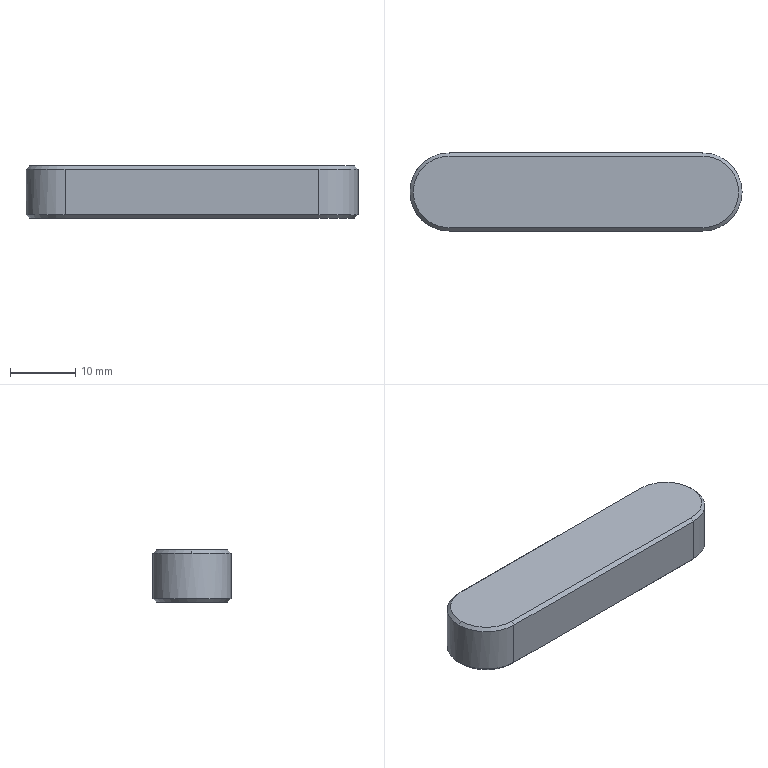Part | SolidWorks | features BaseBody 1 | 1 solid | 17 faces | box 51 x 12 x 8 mm | volume 4620 mm3 | plane 8 | cone 6 | cylinder 3 | commonest cylinder face diameters 12 x3
STEP:
#1=CARTESIAN_POINT('',(29.272,3.607,0.));
#2=VERTEX_POINT('',#1);
#3=CARTESIAN_POINT('',(34.772,9.107,0.));
#4=VERTEX_POINT('',#3);
#5=CARTESIAN_POINT('',(29.272,9.107,0.));
#6=DIRECTION('',(0.,0.,1.));
#7=DIRECTION('',(1.,0.,0.));
#8=AXIS2_PLACEMENT_3D('',#5,#6,#7);
#9=CIRCLE('',#8,5.5);
#10=EDGE_CURVE('',#2,#4,#9,.T.);
#11=ORIENTED_EDGE('',*,*,#10,.T.);
#12=CARTESIAN_POINT('',(35.272,9.107,0.5));
#13=VERTEX_POINT('',#12);
#14=CARTESIAN_POINT('',(35.272,9.107,0.5));
#15=DIRECTION('',(0.7071,0.,0.7071));
#16=VECTOR('',#15,1000.);
#17=LINE('',#14,#16);
#18=EDGE_CURVE('',#4,#13,#17,.T.);
#19=ORIENTED_EDGE('',*,*,#18,.T.);
#20=CARTESIAN_POINT('',(29.272,3.107,0.5));
#21=VERTEX_POINT('',#20);
#22=CARTESIAN_POINT('',(29.272,9.107,0.5));
#23=DIRECTION('',(0.,0.,-1.));
#24=DIRECTION('',(0.,1.,0.));
#25=AXIS2_PLACEMENT_3D('',#22,#23,#24);
#26=CIRCLE('',#25,6.);
#27=EDGE_CURVE('',#13,#21,#26,.T.);
#28=ORIENTED_EDGE('',*,*,#27,.T.);
#29=CARTESIAN_POINT('',(29.272,3.357,0.25));
#30=DIRECTION('',(0.,-0.7071,0.7071));
#31=VECTOR('',#30,1000.);
#32=LINE('',#29,#31);
#33=EDGE_CURVE('',#2,#21,#32,.T.);
#34=ORIENTED_EDGE('',*,*,#33,.F.);
#35=EDGE_LOOP('',(#11,#19,#28,#34));
#36=FACE_OUTER_BOUND('',#35,.T.);
#37=CARTESIAN_POINT('',(29.272,9.107,0.5));
#38=DIRECTION('',(0.,0.,1.));
#39=DIRECTION('',(1.,0.,0.));
#40=AXIS2_PLACEMENT_3D('',#37,#38,#39);
#41=CONICAL_SURFACE('',#40,6.,0.7854);
#42=ADVANCED_FACE('',(#36),#41,.T.);
#43=ORIENTED_EDGE('',*,*,#27,.F.);
#44=CARTESIAN_POINT('',(35.272,9.107,7.5));
#45=VERTEX_POINT('',#44);
#46=CARTESIAN_POINT('',(35.272,9.107,0.));
#47=DIRECTION('',(0.,0.,1.));
#48=VECTOR('',#47,1000.);
#49=LINE('',#46,#48);
#50=EDGE_CURVE('',#13,#45,#49,.T.);
#51=ORIENTED_EDGE('',*,*,#50,.T.);
#52=CARTESIAN_POINT('',(29.272,3.107,7.5));
#53=VERTEX_POINT('',#52);
#54=CARTESIAN_POINT('',(29.272,9.107,7.5));
#55=DIRECTION('',(0.,0.,-1.));
#56=DIRECTION('',(1.,0.,0.));
#57=AXIS2_PLACEMENT_3D('',#54,#55,#56);
#58=CIRCLE('',#57,6.);
#59=EDGE_CURVE('',#45,#53,#58,.T.);
#60=ORIENTED_EDGE('',*,*,#59,.T.);
#61=CARTESIAN_POINT('',(29.272,3.107,0.));
#62=DIRECTION('',(0.,0.,1.));
#63=VECTOR('',#62,1000.);
#64=LINE('',#61,#63);
#65=EDGE_CURVE('',#21,#53,#64,.T.);
#66=ORIENTED_EDGE('',*,*,#65,.F.);
#67=EDGE_LOOP('',(#43,#51,#60,#66));
#68=FACE_OUTER_BOUND('',#67,.T.);
#69=CARTESIAN_POINT('',(29.272,9.107,0.));
#70=DIRECTION('',(0.,0.,1.));
#71=DIRECTION('',(1.,0.,0.));
#72=AXIS2_PLACEMENT_3D('',#69,#70,#71);
#73=CYLINDRICAL_SURFACE('',#72,6.);
#74=ADVANCED_FACE('',(#68),#73,.T.);
#75=CARTESIAN_POINT('',(-9.728,3.607,8.));
#76=VERTEX_POINT('',#75);
#77=CARTESIAN_POINT('',(-15.228,9.107,8.));
#78=VERTEX_POINT('',#77);
#79=CARTESIAN_POINT('',(-9.728,9.107,8.));
#80=DIRECTION('',(0.,0.,-1.));
#81=DIRECTION('',(-1.,0.,0.));
#82=AXIS2_PLACEMENT_3D('',#79,#80,#81);
#83=CIRCLE('',#82,5.5);
#84=EDGE_CURVE('',#76,#78,#83,.T.);
#85=ORIENTED_EDGE('',*,*,#84,.T.);
#86=CARTESIAN_POINT('',(-15.728,9.107,7.5));
#87=VERTEX_POINT('',#86);
#88=CARTESIAN_POINT('',(-15.728,9.107,7.5));
#89=DIRECTION('',(-0.7071,0.,-0.7071));
#90=VECTOR('',#89,1000.);
#91=LINE('',#88,#90);
#92=EDGE_CURVE('',#78,#87,#91,.T.);
#93=ORIENTED_EDGE('',*,*,#92,.T.);
#94=CARTESIAN_POINT('',(-9.728,3.107,7.5));
#95=VERTEX_POINT('',#94);
#96=CARTESIAN_POINT('',(-9.728,9.107,7.5));
#97=DIRECTION('',(0.,0.,-1.));
#98=DIRECTION('',(1.,0.,0.));
#99=AXIS2_PLACEMENT_3D('',#96,#97,#98);
#100=CIRCLE('',#99,6.);
#101=EDGE_CURVE('',#95,#87,#100,.T.);
#102=ORIENTED_EDGE('',*,*,#101,.F.);
#103=CARTESIAN_POINT('',(-9.728,3.357,7.75));
#104=DIRECTION('',(0.,-0.7071,-0.7071));
#105=VECTOR('',#104,1000.);
#106=LINE('',#103,#105);
#107=EDGE_CURVE('',#76,#95,#106,.T.);
#108=ORIENTED_EDGE('',*,*,#107,.F.);
#109=EDGE_LOOP('',(#85,#93,#102,#108));
#110=FACE_OUTER_BOUND('',#109,.T.);
#111=CARTESIAN_POINT('',(-9.728,9.107,7.5));
#112=DIRECTION('',(0.,0.,-1.));
#113=DIRECTION('',(-1.,0.,0.));
#114=AXIS2_PLACEMENT_3D('',#111,#112,#113);
#115=CONICAL_SURFACE('',#114,6.,0.7854);
#116=ADVANCED_FACE('',(#110),#115,.T.);
#117=CARTESIAN_POINT('',(-9.728,14.607,0.));
#118=VERTEX_POINT('',#117);
#119=CARTESIAN_POINT('',(-9.728,3.607,0.));
#120=VERTEX_POINT('',#119);
#121=CARTESIAN_POINT('',(-9.728,9.107,0.));
#122=DIRECTION('',(0.,0.,1.));
#123=DIRECTION('',(1.,0.,0.));
#124=AXIS2_PLACEMENT_3D('',#121,#122,#123);
#125=CIRCLE('',#124,5.5);
#126=EDGE_CURVE('',#118,#120,#125,.T.);
#127=ORIENTED_EDGE('',*,*,#126,.F.);
#128=CARTESIAN_POINT('',(29.272,14.607,0.));
#129=VERTEX_POINT('',#128);
#130=CARTESIAN_POINT('',(9.772,14.607,0.));
#131=DIRECTION('',(-1.,0.,0.));
#132=VECTOR('',#131,1000.);
#133=LINE('',#130,#132);
#134=EDGE_CURVE('',#129,#118,#133,.T.);
#135=ORIENTED_EDGE('',*,*,#134,.F.);
#136=CARTESIAN_POINT('',(29.272,9.107,0.));
#137=DIRECTION('',(0.,0.,1.));
#138=DIRECTION('',(1.,0.,0.));
#139=AXIS2_PLACEMENT_3D('',#136,#137,#138);
#140=CIRCLE('',#139,5.5);
#141=EDGE_CURVE('',#4,#129,#140,.T.);
#142=ORIENTED_EDGE('',*,*,#141,.F.);
#143=ORIENTED_EDGE('',*,*,#10,.F.);
#144=CARTESIAN_POINT('',(9.772,3.607,0.));
#145=DIRECTION('',(1.,0.,0.));
#146=VECTOR('',#145,1000.);
#147=LINE('',#144,#146);
#148=EDGE_CURVE('',#120,#2,#147,.T.);
#149=ORIENTED_EDGE('',*,*,#148,.F.);
#150=EDGE_LOOP('',(#127,#135,#142,#143,#149));
#151=FACE_OUTER_BOUND('',#150,.T.);
#152=CARTESIAN_POINT('',(9.772,9.107,0.));
#153=DIRECTION('',(0.,0.,1.));
#154=DIRECTION('',(1.,0.,0.));
#155=AXIS2_PLACEMENT_3D('',#152,#153,#154);
#156=PLANE('',#155);
#157=ADVANCED_FACE('',(#151),#156,.F.);
#158=CARTESIAN_POINT('',(-9.728,3.107,0.5));
#159=VERTEX_POINT('',#158);
#160=CARTESIAN_POINT('',(-9.728,3.357,0.25));
#161=DIRECTION('',(0.,0.7071,-0.7071));
#162=VECTOR('',#161,1000.);
#163=LINE('',#160,#162);
#164=EDGE_CURVE('',#159,#120,#163,.T.);
#165=ORIENTED_EDGE('',*,*,#164,.T.);
#166=ORIENTED_EDGE('',*,*,#148,.T.);
#167=ORIENTED_EDGE('',*,*,#33,.T.);
#168=CARTESIAN_POINT('',(19.522,3.107,0.5));
#169=DIRECTION('',(-1.,0.,0.));
#170=VECTOR('',#169,1000.);
#171=LINE('',#168,#170);
#172=EDGE_CURVE('',#21,#159,#171,.T.);
#173=ORIENTED_EDGE('',*,*,#172,.T.);
#174=EDGE_LOOP('',(#165,#166,#167,#173));
#175=FACE_OUTER_BOUND('',#174,.T.);
#176=CARTESIAN_POINT('',(19.522,3.357,0.25));
#177=DIRECTION('',(0.,-0.7071,-0.7071));
#178=DIRECTION('',(0.,0.7071,-0.7071));
#179=AXIS2_PLACEMENT_3D('',#176,#177,#178);
#180=PLANE('',#179);
#181=ADVANCED_FACE('',(#175),#180,.T.);
#182=ORIENTED_EDGE('',*,*,#164,.F.);
#183=CARTESIAN_POINT('',(-9.728,15.107,0.5));
#184=VERTEX_POINT('',#183);
#185=CARTESIAN_POINT('',(-9.728,9.107,0.5));
#186=DIRECTION('',(0.,0.,-1.));
#187=DIRECTION('',(0.,-1.,0.));
#188=AXIS2_PLACEMENT_3D('',#185,#186,#187);
#189=CIRCLE('',#188,6.);
#190=EDGE_CURVE('',#159,#184,#189,.T.);
#191=ORIENTED_EDGE('',*,*,#190,.T.);
#192=CARTESIAN_POINT('',(-9.728,499014.607,499000.));
#193=DIRECTION('',(0.,-0.7071,-0.7071));
#194=VECTOR('',#193,1000.);
#195=LINE('',#192,#194);
#196=EDGE_CURVE('',#184,#118,#195,.T.);
#197=ORIENTED_EDGE('',*,*,#196,.T.);
#198=ORIENTED_EDGE('',*,*,#126,.T.);
#199=EDGE_LOOP('',(#182,#191,#197,#198));
#200=FACE_OUTER_BOUND('',#199,.T.);
#201=CARTESIAN_POINT('',(-9.728,9.107,0.5));
#202=DIRECTION('',(0.,0.,1.));
#203=DIRECTION('',(1.,0.,0.));
#204=AXIS2_PLACEMENT_3D('',#201,#202,#203);
#205=CONICAL_SURFACE('',#204,6.,0.7854);
#206=ADVANCED_FACE('',(#200),#205,.T.);
#207=ORIENTED_EDGE('',*,*,#196,.F.);
#208=CARTESIAN_POINT('',(29.272,15.107,0.5));
#209=VERTEX_POINT('',#208);
#210=CARTESIAN_POINT('',(0.02162,15.107,0.5));
#211=DIRECTION('',(1.,0.,0.));
#212=VECTOR('',#211,1000.);
#213=LINE('',#210,#212);
#214=EDGE_CURVE('',#184,#209,#213,.T.);
#215=ORIENTED_EDGE('',*,*,#214,.T.);
#216=CARTESIAN_POINT('',(29.272,14.857,0.25));
#217=DIRECTION('',(0.,-0.7071,-0.7071));
#218=VECTOR('',#217,1000.);
#219=LINE('',#216,#218);
#220=EDGE_CURVE('',#209,#129,#219,.T.);
#221=ORIENTED_EDGE('',*,*,#220,.T.);
#222=ORIENTED_EDGE('',*,*,#134,.T.);
#223=EDGE_LOOP('',(#207,#215,#221,#222));
#224=FACE_OUTER_BOUND('',#223,.T.);
#225=CARTESIAN_POINT('',(0.02162,14.857,0.25));
#226=DIRECTION('',(0.,0.7071,-0.7071));
#227=DIRECTION('',(0.,0.7071,0.7071));
#228=AXIS2_PLACEMENT_3D('',#225,#226,#227);
#229=PLANE('',#228);
#230=ADVANCED_FACE('',(#224),#229,.T.);
#231=ORIENTED_EDGE('',*,*,#18,.F.);
#232=ORIENTED_EDGE('',*,*,#141,.T.);
#233=ORIENTED_EDGE('',*,*,#220,.F.);
#234=CARTESIAN_POINT('',(29.272,9.107,0.5));
#235=DIRECTION('',(0.,0.,-1.));
#236=DIRECTION('',(0.,1.,0.));
#237=AXIS2_PLACEMENT_3D('',#234,#235,#236);
#238=CIRCLE('',#237,6.);
#239=EDGE_CURVE('',#209,#13,#238,.T.);
#240=ORIENTED_EDGE('',*,*,#239,.T.);
#241=EDGE_LOOP('',(#231,#232,#233,#240));
#242=FACE_OUTER_BOUND('',#241,.T.);
#243=CARTESIAN_POINT('',(29.272,9.107,0.5));
#244=DIRECTION('',(0.,0.,1.));
#245=DIRECTION('',(1.,0.,0.));
#246=AXIS2_PLACEMENT_3D('',#243,#244,#245);
#247=CONICAL_SURFACE('',#246,6.,0.7854);
#248=ADVANCED_FACE('',(#242),#247,.T.);
#249=CARTESIAN_POINT('',(29.272,3.107,7.5));
#250=DIRECTION('',(-1.,0.,0.));
#251=VECTOR('',#250,1000.);
#252=LINE('',#249,#251);
#253=EDGE_CURVE('',#53,#95,#252,.T.);
#254=ORIENTED_EDGE('',*,*,#253,.T.);
#255=CARTESIAN_POINT('',(-9.728,3.107,0.));
#256=DIRECTION('',(0.,0.,-1.));
#257=VECTOR('',#256,1000.);
#258=LINE('',#255,#257);
#259=EDGE_CURVE('',#95,#159,#258,.T.);
#260=ORIENTED_EDGE('',*,*,#259,.T.);
#261=ORIENTED_EDGE('',*,*,#172,.F.);
#262=ORIENTED_EDGE('',*,*,#65,.T.);
#263=EDGE_LOOP('',(#254,#260,#261,#262));
#264=FACE_OUTER_BOUND('',#263,.T.);
#265=CARTESIAN_POINT('',(29.272,3.107,0.));
#266=DIRECTION('',(0.,-1.,0.));
#267=DIRECTION('',(0.,0.,-1.));
#268=AXIS2_PLACEMENT_3D('',#265,#266,#267);
#269=PLANE('',#268);
#270=ADVANCED_FACE('',(#264),#269,.T.);
#271=ORIENTED_EDGE('',*,*,#101,.T.);
#272=CARTESIAN_POINT('',(-9.728,15.107,7.5));
#273=VERTEX_POINT('',#272);
#274=CARTESIAN_POINT('',(-9.728,9.107,7.5));
#275=DIRECTION('',(0.,0.,-1.));
#276=DIRECTION('',(1.,0.,0.));
#277=AXIS2_PLACEMENT_3D('',#274,#275,#276);
#278=CIRCLE('',#277,6.);
#279=EDGE_CURVE('',#87,#273,#278,.T.);
#280=ORIENTED_EDGE('',*,*,#279,.T.);
#281=CARTESIAN_POINT('',(-9.728,15.107,0.));
#282=DIRECTION('',(0.,0.,-1.));
#283=VECTOR('',#282,1000.);
#284=LINE('',#281,#283);
#285=EDGE_CURVE('',#273,#184,#284,.T.);
#286=ORIENTED_EDGE('',*,*,#285,.T.);
#287=ORIENTED_EDGE('',*,*,#190,.F.);
#288=ORIENTED_EDGE('',*,*,#259,.F.);
#289=EDGE_LOOP('',(#271,#280,#286,#287,#288));
#290=FACE_OUTER_BOUND('',#289,.T.);
#291=CARTESIAN_POINT('',(-9.728,9.107,0.));
#292=DIRECTION('',(0.,0.,1.));
#293=DIRECTION('',(1.,0.,0.));
#294=AXIS2_PLACEMENT_3D('',#291,#292,#293);
#295=CYLINDRICAL_SURFACE('',#294,6.);
#296=ADVANCED_FACE('',(#290),#295,.T.);
#297=CARTESIAN_POINT('',(29.272,15.107,7.5));
#298=VERTEX_POINT('',#297);
#299=CARTESIAN_POINT('',(-9.728,15.107,7.5));
#300=DIRECTION('',(1.,0.,0.));
#301=VECTOR('',#300,1000.);
#302=LINE('',#299,#301);
#303=EDGE_CURVE('',#273,#298,#302,.T.);
#304=ORIENTED_EDGE('',*,*,#303,.T.);
#305=CARTESIAN_POINT('',(29.272,15.107,0.));
#306=DIRECTION('',(0.,0.,-1.));
#307=VECTOR('',#306,1000.);
#308=LINE('',#305,#307);
#309=EDGE_CURVE('',#298,#209,#308,.T.);
#310=ORIENTED_EDGE('',*,*,#309,.T.);
#311=ORIENTED_EDGE('',*,*,#214,.F.);
#312=ORIENTED_EDGE('',*,*,#285,.F.);
#313=EDGE_LOOP('',(#304,#310,#311,#312));
#314=FACE_OUTER_BOUND('',#313,.T.);
#315=CARTESIAN_POINT('',(-9.728,15.107,0.));
#316=DIRECTION('',(0.,1.,0.));
#317=DIRECTION('',(0.,0.,1.));
#318=AXIS2_PLACEMENT_3D('',#315,#316,#317);
#319=PLANE('',#318);
#320=ADVANCED_FACE('',(#314),#319,.T.);
#321=ORIENTED_EDGE('',*,*,#50,.F.);
#322=ORIENTED_EDGE('',*,*,#239,.F.);
#323=ORIENTED_EDGE('',*,*,#309,.F.);
#324=CARTESIAN_POINT('',(29.272,9.107,7.5));
#325=DIRECTION('',(0.,0.,-1.));
#326=DIRECTION('',(1.,0.,0.));
#327=AXIS2_PLACEMENT_3D('',#324,#325,#326);
#328=CIRCLE('',#327,6.);
#329=EDGE_CURVE('',#298,#45,#328,.T.);
#330=ORIENTED_EDGE('',*,*,#329,.T.);
#331=EDGE_LOOP('',(#321,#322,#323,#330));
#332=FACE_OUTER_BOUND('',#331,.T.);
#333=CARTESIAN_POINT('',(29.272,9.107,0.));
#334=DIRECTION('',(0.,0.,1.));
#335=DIRECTION('',(1.,0.,0.));
#336=AXIS2_PLACEMENT_3D('',#333,#334,#335);
#337=CYLINDRICAL_SURFACE('',#336,6.);
#338=ADVANCED_FACE('',(#332),#337,.T.);
#339=ORIENTED_EDGE('',*,*,#107,.T.);
#340=ORIENTED_EDGE('',*,*,#253,.F.);
#341=CARTESIAN_POINT('',(29.272,3.607,8.));
#342=VERTEX_POINT('',#341);
#343=CARTESIAN_POINT('',(29.272,3.357,7.75));
#344=DIRECTION('',(0.,0.7071,0.7071));
#345=VECTOR('',#344,1000.);
#346=LINE('',#343,#345);
#347=EDGE_CURVE('',#53,#342,#346,.T.);
#348=ORIENTED_EDGE('',*,*,#347,.T.);
#349=CARTESIAN_POINT('',(19.522,3.607,8.));
#350=DIRECTION('',(-1.,0.,0.));
#351=VECTOR('',#350,1000.);
#352=LINE('',#349,#351);
#353=EDGE_CURVE('',#342,#76,#352,.T.);
#354=ORIENTED_EDGE('',*,*,#353,.T.);
#355=EDGE_LOOP('',(#339,#340,#348,#354));
#356=FACE_OUTER_BOUND('',#355,.T.);
#357=CARTESIAN_POINT('',(19.522,3.357,7.75));
#358=DIRECTION('',(0.,-0.7071,0.7071));
#359=DIRECTION('',(0.,-0.7071,-0.7071));
#360=AXIS2_PLACEMENT_3D('',#357,#358,#359);
#361=PLANE('',#360);
#362=ADVANCED_FACE('',(#356),#361,.T.);
#363=ORIENTED_EDGE('',*,*,#92,.F.);
#364=CARTESIAN_POINT('',(-9.728,14.607,8.));
#365=VERTEX_POINT('',#364);
#366=CARTESIAN_POINT('',(-9.728,9.107,8.));
#367=DIRECTION('',(0.,0.,-1.));
#368=DIRECTION('',(-1.,0.,0.));
#369=AXIS2_PLACEMENT_3D('',#366,#367,#368);
#370=CIRCLE('',#369,5.5);
#371=EDGE_CURVE('',#78,#365,#370,.T.);
#372=ORIENTED_EDGE('',*,*,#371,.T.);
#373=CARTESIAN_POINT('',(-9.728,499018.214,-498995.607));
#374=DIRECTION('',(0.,0.7071,-0.7071));
#375=VECTOR('',#374,1000.);
#376=LINE('',#373,#375);
#377=EDGE_CURVE('',#365,#273,#376,.T.);
#378=ORIENTED_EDGE('',*,*,#377,.T.);
#379=ORIENTED_EDGE('',*,*,#279,.F.);
#380=EDGE_LOOP('',(#363,#372,#378,#379));
#381=FACE_OUTER_BOUND('',#380,.T.);
#382=CARTESIAN_POINT('',(-9.728,9.107,7.5));
#383=DIRECTION('',(0.,0.,-1.));
#384=DIRECTION('',(-1.,0.,0.));
#385=AXIS2_PLACEMENT_3D('',#382,#383,#384);
#386=CONICAL_SURFACE('',#385,6.,0.7854);
#387=ADVANCED_FACE('',(#381),#386,.T.);
#388=ORIENTED_EDGE('',*,*,#377,.F.);
#389=CARTESIAN_POINT('',(29.272,14.607,8.));
#390=VERTEX_POINT('',#389);
#391=CARTESIAN_POINT('',(0.02162,14.607,8.));
#392=DIRECTION('',(1.,0.,0.));
#393=VECTOR('',#392,1000.);
#394=LINE('',#391,#393);
#395=EDGE_CURVE('',#365,#390,#394,.T.);
#396=ORIENTED_EDGE('',*,*,#395,.T.);
#397=CARTESIAN_POINT('',(29.272,14.857,7.75));
#398=DIRECTION('',(0.,0.7071,-0.7071));
#399=VECTOR('',#398,1000.);
#400=LINE('',#397,#399);
#401=EDGE_CURVE('',#390,#298,#400,.T.);
#402=ORIENTED_EDGE('',*,*,#401,.T.);
#403=ORIENTED_EDGE('',*,*,#303,.F.);
#404=EDGE_LOOP('',(#388,#396,#402,#403));
#405=FACE_OUTER_BOUND('',#404,.T.);
#406=CARTESIAN_POINT('',(0.02162,14.857,7.75));
#407=DIRECTION('',(0.,0.7071,0.7071));
#408=DIRECTION('',(0.,-0.7071,0.7071));
#409=AXIS2_PLACEMENT_3D('',#406,#407,#408);
#410=PLANE('',#409);
#411=ADVANCED_FACE('',(#405),#410,.T.);
#412=ORIENTED_EDGE('',*,*,#347,.F.);
#413=ORIENTED_EDGE('',*,*,#59,.F.);
#414=ORIENTED_EDGE('',*,*,#329,.F.);
#415=ORIENTED_EDGE('',*,*,#401,.F.);
#416=CARTESIAN_POINT('',(29.272,9.107,8.));
#417=DIRECTION('',(0.,0.,-1.));
#418=DIRECTION('',(-1.,0.,0.));
#419=AXIS2_PLACEMENT_3D('',#416,#417,#418);
#420=CIRCLE('',#419,5.5);
#421=EDGE_CURVE('',#390,#342,#420,.T.);
#422=ORIENTED_EDGE('',*,*,#421,.T.);
#423=EDGE_LOOP('',(#412,#413,#414,#415,#422));
#424=FACE_OUTER_BOUND('',#423,.T.);
#425=CARTESIAN_POINT('',(29.272,9.107,7.5));
#426=DIRECTION('',(0.,0.,-1.));
#427=DIRECTION('',(-1.,0.,0.));
#428=AXIS2_PLACEMENT_3D('',#425,#426,#427);
#429=CONICAL_SURFACE('',#428,6.,0.7854);
#430=ADVANCED_FACE('',(#424),#429,.T.);
#431=ORIENTED_EDGE('',*,*,#395,.F.);
#432=ORIENTED_EDGE('',*,*,#371,.F.);
#433=ORIENTED_EDGE('',*,*,#84,.F.);
#434=ORIENTED_EDGE('',*,*,#353,.F.);
#435=ORIENTED_EDGE('',*,*,#421,.F.);
#436=EDGE_LOOP('',(#431,#432,#433,#434,#435));
#437=FACE_OUTER_BOUND('',#436,.T.);
#438=CARTESIAN_POINT('',(9.772,9.107,8.));
#439=DIRECTION('',(0.,0.,1.));
#440=DIRECTION('',(1.,0.,0.));
#441=AXIS2_PLACEMENT_3D('',#438,#439,#440);
#442=PLANE('',#441);
#443=ADVANCED_FACE('',(#437),#442,.T.);
#444=CLOSED_SHELL('',(#42,#74,#116,#157,#181,#206,#230,#248,#270,#296,#320,#338,#362,#387,#411,#430,#443));
#445=MANIFOLD_SOLID_BREP('',#444);
#446=CARTESIAN_POINT('',(0.,0.,0.));
#447=DIRECTION('',(0.,0.,1.));
#448=DIRECTION('',(1.,0.,0.));
#449=AXIS2_PLACEMENT_3D('',#446,#447,#448);
#450=(LENGTH_UNIT()NAMED_UNIT(*)SI_UNIT(.MILLI.,.METRE.));
#451=UNCERTAINTY_MEASURE_WITH_UNIT(LENGTH_MEASURE(0.00001),#450,'','');
#452=(NAMED_UNIT(*)PLANE_ANGLE_UNIT()SI_UNIT($,.RADIAN.));
#453=(NAMED_UNIT(*)SI_UNIT($,.STERADIAN.)SOLID_ANGLE_UNIT());
#454=(GEOMETRIC_REPRESENTATION_CONTEXT(3)GLOBAL_UNCERTAINTY_ASSIGNED_CONTEXT((#451))GLOBAL_UNIT_ASSIGNED_CONTEXT((#450,#452,#453))REPRESENTATION_CONTEXT('',''));
#455=ADVANCED_BREP_SHAPE_REPRESENTATION('',(#445,#449),#454);